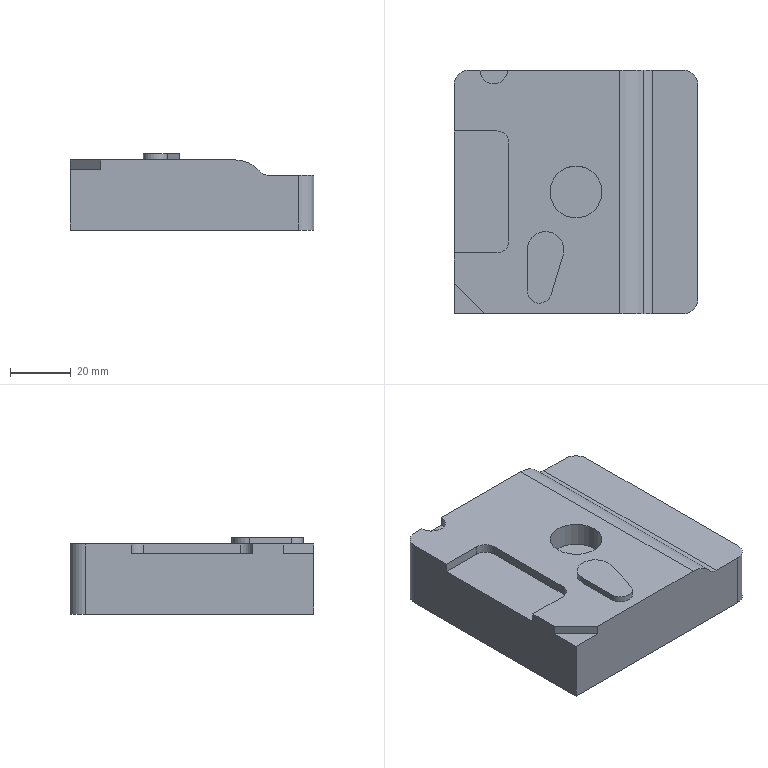CAM job | NX | 3-axis milling | part box 80 x 80 x 25 mm | stock box 80 x 80 x 25 mm
Tools:
number,name,description,diameter,corner_radius,flute_length,length,flutes
0,D6,Milling Tool-5 Parameters,6.0,0.0,50.0,75.0,2
0,D12D,Milling Tool-5 Parameters,12.0,0.0,50.0,75.0,2
0,B6,Milling Tool-Ball Mill,6.0,3.0,50.0,75.0,2
Operations:
program,operation,operation_type,tool,method,geometry_group,spindle_rpm,surface_speed,feed_per_tooth,feed_cut,feed_plunge,cut_length_mm,path_length_mm,cut_time_min,machine_time_min
NC_PROGRAM,CAVITY_MILL,CavityMilling,D12D,MILL_ROUGH,WORKPIECE,0.0,0.0,0.0,250.0,100.0,15609.845,23482.103,62.439,63.227
NC_PROGRAM,REST_MILLING,CavityMilling,D6,MILL_ROUGH,WORKPIECE,0.0,0.0,0.0,250.0,100.0,20282.909,37440.612,81.132,82.847
NC_PROGRAM,FACE_MILLING_AREA,VolumeBased25DMillingOperation,D6,MILL_FINISH,WORKPIECE,0.0,0.0,0.0,250.0,100.0,2146.746,2244.979,8.587,8.597
NC_PROGRAM,FIXED_CONTOUR,SurfaceContour,B6,MILL_FINISH,WORKPIECE,0.0,0.0,0.0,250.0,100.0,981.577,996.573,3.926,3.928
NC_PROGRAM,PLANAR_PROFILE,PlanarMilling,D6,METHOD,WORKPIECE,0.0,0.0,0.0,250.0,100.0,347.836,403.836,1.391,1.397